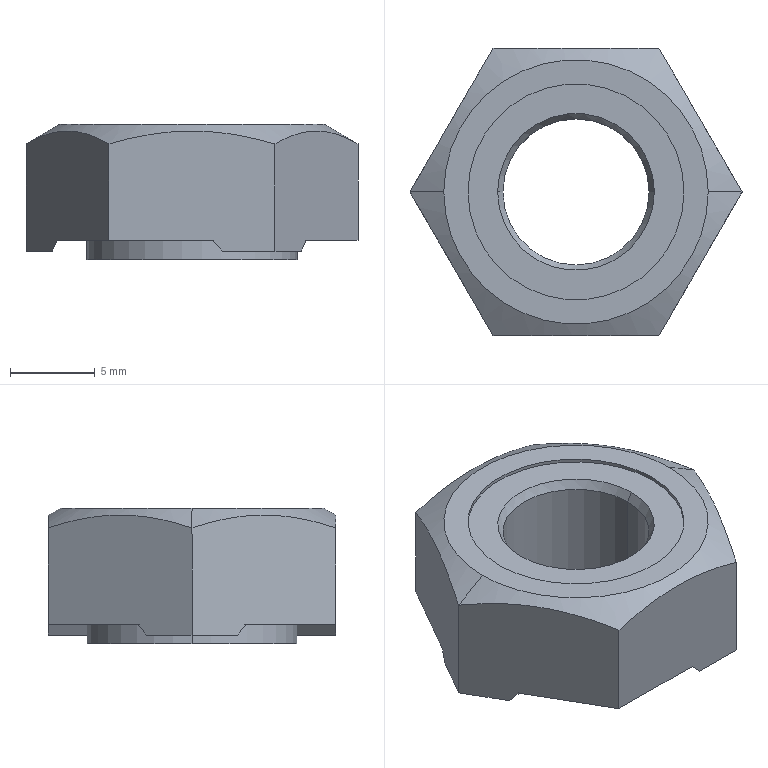Part | STEP file | hexagon weld nuts gb_GB_FASTENER_NUT_JSCN M10X1.25-N | 1 solid | 28 faces | box 19.63 x 17 x 8 mm | volume 1354 mm3 | plane 16 | cone 6 | cylinder 6 | commonest cylinder face diameters 8.647 x2 12.45 x2 12.77 x2